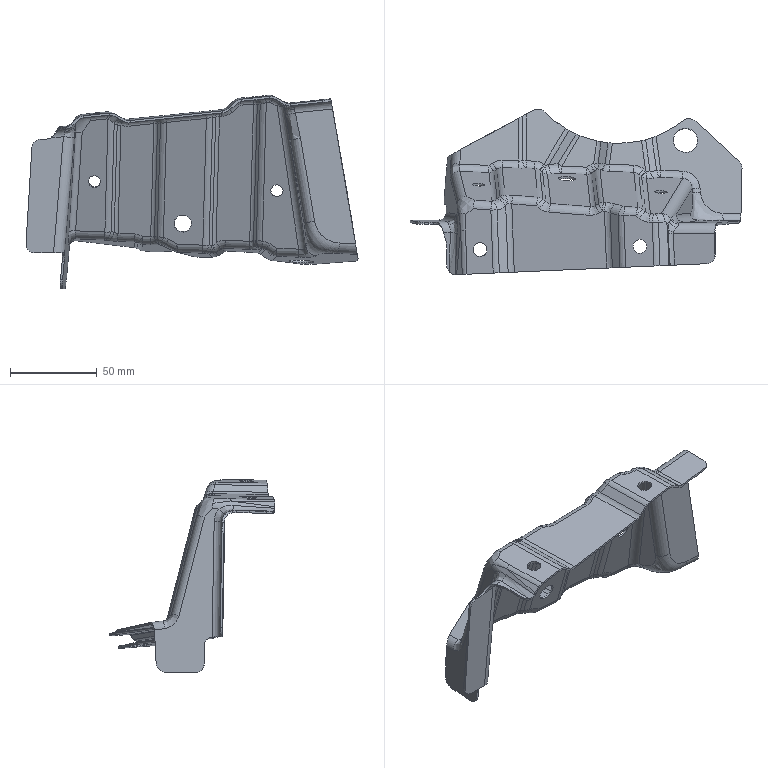Part | 1 solid | 358 faces | box 190.934 x 95.254 x 111.136 mm | volume 32051 mm3 | spline 167 | cylinder 126 | plane 39 | sphere 24 | other 2 | commonest cylinder face diameters 10 x49 12.4 x24 7.6 x23 12 x9 9.6 x6 7 x4